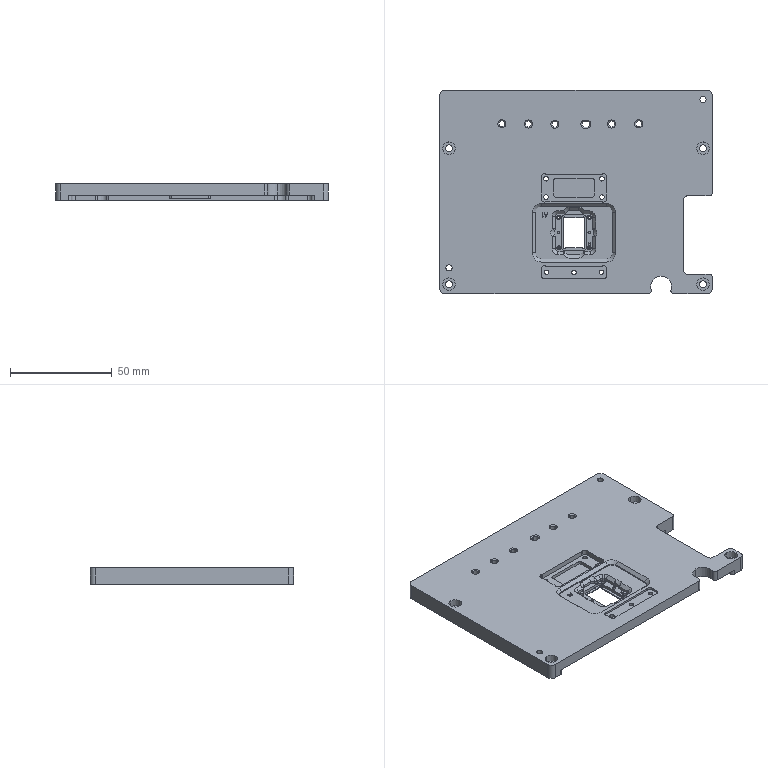NC program | NX | posted with a generic post | part box 134 x 100 x 8 mm
Lines 1 to 1315 of 16793:
N10 G17 G21 G94 G90
(FLOOR_WALL_COPY , TOOL : D63)
N12 T03 M6
N14 G54
N16 G17 G0 G90 X-105.5 Y53.999 S6500 M3
N18 G43 Z30. H3
N20 Z3.
N22 G94 G1 Z0. F1250.
N24 X-102.5
N26 X102.5
N28 Y12.6
N30 X-102.5
N32 Y-28.8
N34 X102.5
N36 X105.5
N38 Z3.
N40 G0 Z30.
N42 M5
(DRILLING_COPY_1 , TOOL : D6A45)
N44 T01 M6
N46 G54
N48 G17 G0 G90 X-62.5 Y-45.396 S5000 M3
N50 G43 Z30. H1
N52 G94 G81 G98 Z-0.5 F250. R3.
N54 Y-37.296
N56 Y21.5
N58 X-36.457 Y33.557
N60 X-23.437 Y33.443
N62 X-10.372 Y33.331
N64 X4.356
N66 X17.491 Y33.445
N68 X30.853 Y33.52
N70 X62.5 Y45.5
N72 Y21.5
N74 X12.75 Y6.5
N76 Y-2.5
N78 X-14.75 Y6.5
N80 Y-2.5
N82 X-8.5 Y-12.5
N84 X-5.7 Y-12.88
N86 X3.7
N88 X6.5 Y-12.5
N90 Y-27.5
N92 X3.7 Y-27.12
N94 X-5.7
N96 X-8.5 Y-27.5
N98 X-14.5 Y-39.5
N100 X-1.
N102 X12.5
N104 X62.5 Y-45.396
N106 G80
N108 G0 X62.5 Y-45.396 Z30.
N110 M5
(DRILLING_COPY_1_COPY , TOOL : 3.5ZT)
N112 T13 M6
N114 G54
N116 G17 G0 G90 X-62.5 Y21.5 S2000 M3
N118 G43 Z30. H13
N120 G94 G83 G98 Z-10.552 F150. Q2. R3.
N122 Y-45.396
N124 X62.5
N126 Y21.5
N128 G80
N130 G0 X62.5 Y21.5 Z30.
N132 M5
(DRILLING_COPY_1_COPY_COPY , TOOL : 2.2ZT)
N134 T12 M6
N136 G54
N138 G17 G0 G90 X-62.5 Y-37.296 S2000 M3
N140 G43 Z30. H12
N142 G94 G83 G98 Z-10.161 F150. Q2. R3.
N144 X-14.5 Y-39.5 Z-4.661
N146 X-1.
N148 X12.5
N150 X12.75 Y-2.5 Z-6.261
N152 Y6.5
N154 X-14.75 Y-2.5
N156 Y6.5
N158 X4.356 Y33.331 Z-7.661
N160 X62.5 Y45.5 Z-10.161
N162 G80
N164 G0 X62.5 Y45.5 Z30.
N166 M5
(DRILLING_COPY_1_COPY_COPY_COPY_2 , TOOL : 3.0ZT)
N168 T23 M6
N170 G54
N172 G17 G0 G90 X-36.457 Y33.557 S2000 M3
N174 G43 Z30. H23
N176 G94 G83 G98 Z-7.901 F150. Q2. R3.
N178 X-23.437 Y33.443
N180 X-10.372 Y33.331
N182 X17.491 Y33.445
N184 X30.853 Y33.52
N186 G80
N188 G0 X30.853 Y33.52 Z30.
N190 M5
(DRILLING_COPY_1_COPY_COPY_COPY , TOOL : 1.0ZT)
N192 T11 M6
N194 G54
N196 G17 G0 G90 X-8.5 Y-12.5 S3000 M3
N198 G43 Z30. H11
N200 G94 G83 G98 Z-8.9 F100. Q1. R3.
N202 X6.5
N204 Y-27.5
N206 X-8.5
N208 G80
N210 G0 X-8.5 Y-27.5 Z30.
N212 M5
(DRILLING_COPY_1_COPY_COPY_COPY_1 , TOOL : 1.2ZT)
N214 T20 M6
N216 G54
N218 G17 G0 G90 X3.7 Y-12.88 S3000 M3
N220 G43 Z30. H20
N222 G94 G83 G98 Z-8.611 F100. Q1. R3.
N224 X-5.7
N226 Y-27.12
N228 X3.7
N230 G80
N232 G0 X3.7 Y-27.12 Z30.
N234 M5
(ADAPTIVE_MILLING_COPY , TOOL : D10)
N236 T04 M6
N238 G54
N240 G17 G0 G90 X-78.709 Y-0.061 S9500 M3
N242 G43 Z30. H4
N244 Z-7.
N246 G94 G1 Z-8. F1000.
N248 X-77.928 Y-0.341 F3500.
N250 X-77.14 Y-0.597
N252 G3 X-76.062 Y-0.061 R1.017
N254 X-75.301 Y3.002 R8.28
N256 X-75.019 Y12.869 R111.643
N258 G1 X-75.014 Y15.119
N260 X-75.011 Y18.994
N262 X-75.01 Y32.619
N264 Y50.869
N266 X-75.009 Y50.994
N268 X-75.008 Y51.119
N270 G2 X-72.514 Y55.4 R5.714
N272 X-66.951 Y57.485 R12.445
N274 X-58.346 Y57.959 R64.172
N276 G1 X-57.221 Y57.968
N278 X-55.721 Y57.976
N280 X-53.846 Y57.982
N282 X-50.971 Y57.985
N284 X-45.096 Y57.987
N286 X68.029 Y57.988
N288 X68.154 Y57.986
N290 X68.279 Y57.979
N292 X68.404 Y57.968
N294 G2 X72.57 Y55.264 R5.937
N296 X74.529 Y49.65 R13.117
N298 X74.964 Y40.792 R70.999
N300 G1 X74.973 Y39.542
N302 X74.979 Y38.042
N304 X74.984 Y35.792
N306 X74.987 Y32.042
N308 X74.988 Y20.292
N310 Y-50.958
N312 G2 X72.718 Y-55.225 R5.577
N314 X67.211 Y-57.439 R11.915
N316 X59.11 Y-57.951 R54.383
N318 G1 X58.235 Y-57.96
N320 X56.985 Y-57.97
N322 X55.735 Y-57.976
N324 X53.86 Y-57.982
N326 X50.86 Y-57.986
N328 X44.36 Y-57.987
N330 X-68.015 Y-57.988
N332 X-68.14 Y-57.986
N334 X-68.265 Y-57.979
N336 X-68.389 Y-57.969
N338 G2 X-72.56 Y-55.274 R5.92
N340 X-74.527 Y-49.661 R13.075
N342 X-74.964 Y-40.804 R70.368
N344 G1 X-74.973 Y-39.554
N346 X-74.979 Y-37.929
N348 X-74.984 Y-35.554
N350 X-74.987 Y-31.554
N352 X-74.988 Y-16.679
N354 Y-3.804
N356 G2 X-74.49 Y1.42 R59.156
N358 G3 X-74.037 Y13.656 R126.306
N360 G1 X-74.031 Y15.406
N362 X-74.025 Y17.906
N364 X-74.022 Y21.906
N366 X-74.021 Y32.906
N368 Y47.906
N370 X-74.019 Y48.031
N372 G2 X-70.421 Y54.267 R7.625
N374 X-64.091 Y56.445 R15.186
N376 X-55.111 Y56.94 R70.872
N378 G1 X-53.986 Y56.951
N380 X-52.611 Y56.96
N382 X-50.861 Y56.967
N384 X-48.486 Y56.972
N386 X-44.611 Y56.976
N388 X-33.111 Y56.977
N390 X64.889
N392 X65.139 Y56.975
N394 X65.264 Y56.97
N396 X65.389 Y56.964
N398 G2 X71.397 Y53.191 R7.687
N400 X73.483 Y46.827 R15.724
N402 X73.952 Y36.844 R83.323
N404 G1 X73.962 Y35.344
N406 X73.969 Y33.344
N408 X73.974 Y30.844
N410 X73.977 Y26.344
N412 Y5.594
N414 X73.978 Y-30.031
N416 X73.984 Y-31.656
N418 X73.983 Y-33.031
N420 X73.987 Y-34.031
N422 X73.984 Y-35.531
N424 X73.987 Y-36.406
N426 X73.986 Y-37.406
N428 X73.989 Y-38.656
N430 X73.987 Y-39.656
N432 X73.988 Y-40.406
N434 X73.987 Y-41.531
N436 X73.986 Y-42.156
N438 X73.988 Y-43.031
N440 X73.986 Y-44.281
N442 X73.988 Y-45.156
N444 X73.987 Y-46.281
N446 X73.99 Y-47.531
N448 X73.989 Y-47.906
N450 X73.986 Y-48.156
N452 X73.981 Y-48.28
N454 X73.974 Y-48.405
N456 G2 X70.182 Y-54.403 R7.71
N458 X63.941 Y-56.47 R15.659
N460 X54.459 Y-56.947 R77.622
N462 G1 X53.209 Y-56.957
N464 X51.584 Y-56.965
N466 X49.584 Y-56.97
N468 X46.459 Y-56.975
N470 X40.334 Y-56.977
N472 X-64.916
N474 X-65.041 Y-56.976
N476 X-65.166 Y-56.973
N478 X-65.291 Y-56.968
N480 X-65.416 Y-56.962
N482 X-65.54 Y-56.953
N484 G2 X-71.411 Y-53.165 R7.74
N486 X-73.503 Y-46.673 R15.948
N488 X-73.956 Y-36.439 R88.425
N490 G1 X-73.964 Y-34.939
N492 X-73.97 Y-33.064
N494 X-73.974 Y-30.314
N496 X-73.977 Y-25.314
N498 Y-6.189
N500 X-73.975 Y-5.814
N502 G2 X-73.436 Y2.041 R136.426
N504 G3 X-73.042 Y17.282 R216.987
N506 G1 X-73.037 Y19.907
N508 X-73.033 Y23.907
N510 X-73.031 Y33.407
N512 Y44.907
N514 X-73.029 Y45.282
N516 X-73.028 Y45.407
N518 G2 X-71.472 Y50.593 R8.925
N520 X-70.439 Y52.312 R10.087
N522 X-67.763 Y54.412 R8.758
N524 X-63.801 Y55.355 R14.165
N526 X-52.823 Y55.929 R91.403
N528 G1 X-51.698 Y55.939
N530 X-50.198 Y55.948
N532 X-48.323 Y55.956
N534 X-45.823 Y55.961
N536 X-41.823 Y55.965
N538 X-31.948 Y55.966
N540 X62.302
N542 X62.552 Y55.963
N544 X62.677 Y55.961
N546 X62.927 Y55.953
N548 X63.052 Y55.947
N550 G2 X67.462 Y54.517 R8.648
N552 G1 X67.763 Y54.412
N554 X67.87 Y54.361
N556 G2 X70.513 Y52.219 R8.758
N558 X72.187 Y47.913 R8.812
N560 X72.917 Y36.948 R74.282
N562 G1 X72.93 Y35.823
N564 X72.941 Y34.573
N566 X72.949 Y33.073
N568 X72.957 Y31.198
N570 X72.962 Y28.573
N572 X72.965 Y24.448
N574 X72.967 Y13.698
N576 Y-26.927
N578 X72.974 Y-28.302
N580 X72.975 Y-30.052
N582 X72.978 Y-30.802
N584 X72.98 Y-31.927
N586 G2 X72.958 Y-46.177 R809.535
N588 X71.503 Y-50.503 R8.675
N590 X70.439 Y-52.312 R8.604
N592 X67.763 Y-54.412 R8.758
N594 X63.801 Y-55.355 R14.165
N596 X52.823 Y-55.93 R91.279
N598 G1 X51.573 Y-55.94
N600 X50.073 Y-55.949
N602 X48.073 Y-55.956
N604 X45.448 Y-55.962
N606 X41.198 Y-55.965
N608 X29.198 Y-55.966
N610 X-62.302
N612 X-62.427 Y-55.965
N614 X-62.552 Y-55.963
N616 X-62.802 Y-55.956
N618 X-62.927 Y-55.951
N620 X-63.052 Y-55.945
N622 G2 X-67.453 Y-54.52 R8.649
N624 G1 X-67.763 Y-54.412
N626 X-67.87 Y-54.361
N628 G2 X-70.513 Y-52.219 R8.758
N630 X-72.187 Y-47.913 R8.812
N632 X-72.908 Y-37.572 R72.544
N634 X-72.966 Y-22.073 R825.905
N636 X-72.913 Y-5.323 R785.834
N638 G1 X-72.893 Y-4.824
N640 X-72.869 Y-4.324
N642 X-72.841 Y-3.825
N644 X-72.81 Y-3.326
N646 X-72.759 Y-2.578
N648 X-72.688 Y-1.58
N650 X-72.597 Y-0.334
N652 X-72.498 Y1.163
N654 X-72.401 Y2.66
N656 X-72.358 Y3.409
N658 X-72.326 Y4.033
N660 X-72.297 Y4.657
N662 X-72.26 Y5.531
N664 X-72.227 Y6.406
N666 X-72.198 Y7.28
N668 X-72.177 Y8.03
N670 X-72.154 Y8.905
N672 X-72.15 Y9.087
N674 Y47.47
N676 X-72.147 Y47.53
N678 X-71.965 Y49.143
N680 X-71.938 Y49.259
N682 X-71.443 Y50.674
N684 G2 X-69.219 Y53.513 R8.407
N686 X-66.143 Y54.965 R8.758
N688 G1 X-64.53 Y55.147
N690 X-64.47 Y55.15
N692 X64.47
N694 X64.53 Y55.147
N696 X66.143 Y54.965
N698 X66.259 Y54.938
N700 X67.556 Y54.484
N702 X67.87 Y54.361
N704 G2 X70.513 Y52.219 R8.758
N706 X71.965 Y49.143 R8.758
N708 G1 X72.147 Y47.53
N710 X72.15 Y47.47
N712 Y-0.401
N714 G3 X71.979 Y-14.083 R281.781
N716 G1 X71.978 Y-23.833
N718 Y-40.458
N720 X71.983 Y-40.513
N722 X71.99 Y-40.544
N724 X72.147 Y-41.935
N726 X72.15 Y-41.994
N728 Y-47.47
N730 X72.147 Y-47.53
N732 X71.965 Y-49.143
N734 X71.938 Y-49.259
N736 X71.484 Y-50.556
N738 G3 X73.623 Y-50.935 R-1.1
N740 G1 X73.776 Y-40.187
N742 X73.804 Y-38.187 Z-7.9
N744 X74.308 Y-2.823
N746 X74.336 Y-0.823 Z-8.
N748 G3 X74.131 Y0.061 R1.327
N750 X72.147 Y-0.461 R1.101
N752 G2 X71.621 Y-3.038 R8.661
N754 G3 X71.061 Y-9.127 R31.238
N756 X70.989 Y-24.377 R776.181
N758 G1 Y-37.877
N760 Y-38.002
N762 X71.002 Y-38.126
N764 G3 X71.511 Y-39.135 R3.65
N766 G1 X71.964 Y-40.428
N768 X71.99 Y-40.544
N770 G3 X73.845 Y-41.071 R1.102
N772 X74.161 Y-40.102 Z-7.947 R1.227
N774 G1 X74.154 Y-39.155 Z-7.9
N776 X73.903 Y-4.015
N778 Y-3.374 Z-7.932
N780 X73.879 Y-2.734 Z-7.964
N782 G3 X73.543 Y-2.114 Z-8. R1.143
N784 X71.757 Y-2.557 R1.102
N786 G2 X71.062 Y-4.145 R11.213
N788 G3 X70.204 Y-9.179 R17.999
N790 X70.004 Y-21.301 R238.834
N792 X70.029 Y-36.425 R855.256
N794 X70.657 Y-37.776 R1.574
N796 G1 X70.731 Y-37.869
N798 X71.13 Y-38.504
N800 G3 X72.608 Y-38.873 R1.104
N802 X73.162 Y-37.83 Z-7.938 R1.124
N804 G1 X73.166 Y-37.074 Z-7.9
N806 X73.353 Y-5.053
N808 X73.347 Y-4.011 Z-7.952
N810 G3 X72.843 Y-3.232 Z-8. R1.117
N812 X71.327 Y-3.579 R1.104
N814 X69.531 Y-8.312 R9.834
N816 X69.046 Y-17.542 R72.207
N818 X69.055 Y-35.041 R637.354
N820 X69.372 Y-36.492 R3.287
N822 G1 X69.448 Y-36.592
N824 X69.533 Y-36.684
N826 X69.578 Y-36.722
N828 X69.596 Y-36.733
N830 X69.688 Y-36.807
N832 X70.395 Y-37.514
N834 G3 X71.725 Y-37.688 R1.108
N836 X72.274 Y-36.655 Z-7.938 R1.125
N838 G1 X72.285 Y-35.887 Z-7.9
N840 X72.679 Y-6.107
N842 X72.681 Y-5.068 Z-7.952
N844 G3 X72.181 Y-4.284 Z-8. R1.117
N846 X70.731 Y-4.527 R1.106
N848 X69.01 Y-7.65 R6.182
N850 X68.163 Y-14.836 R33.413
N852 X68.073 Y-33.709 R409.302
N854 X68.585 Y-36.005 R5.128
N856 X69.596 Y-36.733 R3.984
N858 X70.75 Y-36.743 R1.112
N860 X71.286 Y-35.654 Z-7.936 R1.183
N862 G1 X71.307 Y-34.932 Z-7.9
N864 X72.154 Y-6.662
N866 X72.174 Y-5.624 Z-7.952
N868 G3 X71.685 Y-4.831 Z-8. R1.117
N870 X70.303 Y-4.973 R1.106
N872 X68.11 Y-8.666 R6.798
N874 X67.213 Y-15.72 R32.889
N876 X67.099 Y-32.592 R281.712
N878 X67.726 Y-35.503 R7.4
N880 X68.436 Y-36.004 R1.472
N882 G1 X68.859 Y-36.271
N884 G3 X70.057 Y-36.253 R1.111
N886 X70.547 Y-35.279 Z-7.943 R1.132
N888 G1 X70.575 Y-34.417 Z-7.9
N890 X71.445 Y-7.381
N892 X71.467 Y-6.326 Z-7.953
N894 G3 X70.996 Y-5.541 Z-8. R1.117
N896 X69.688 Y-5.588 R1.108
N898 X67.704 Y-8.074 R4.795
N900 X66.404 Y-14.417 R21.662
N902 X66.061 Y-26.534 R167.955
N904 X66.273 Y-33.025 R47.803
N906 X67.075 Y-35.367 R5.249
N908 X68.288 Y-35.939 R2.889
N910 X69.303 Y-35.786 R1.116
N912 X69.758 Y-34.763 Z-7.942 R1.202
N914 G1 X69.794 Y-33.931 Z-7.9
N916 X70.922 Y-7.779
N918 X70.949 Y-7.222 Z-7.928
N920 X70.956 Y-6.664 Z-7.956
N922 G3 X70.529 Y-5.917 Z-8. R1.128
N924 X69.278 Y-5.862 R1.108
N926 X66.876 Y-8.634 R5.157
N928 X65.496 Y-14.833 R21.41
N930 X65.149 Y-30.57 R145.818
N932 X65.959 Y-34.59 R11.113
N934 X67.036 Y-35.501 R1.403
N936 G1 X67.508 Y-35.666
N938 G3 X68.6 Y-35.451 R1.112
N940 X68.979 Y-34.491 Z-7.947 R1.22
N942 G1 X69.021 Y-33.56 Z-7.9
N944 X70.178 Y-8.255
N946 X70.207 Y-7.695 Z-7.928
N948 X70.215 Y-7.134 Z-7.956
N950 G3 X69.797 Y-6.389 Z-8. R1.128
N952 X68.537 Y-6.327 R1.108
N954 X66.31 Y-8.578 R4.465
N956 X64.687 Y-14.452 R17.91
N958 X64.118 Y-25.556 R98.682
N960 X64.502 Y-32.408 R34.226
N962 X65.688 Y-35.122 R5.464
N964 X66.92 Y-35.474 R2.043
N966 X67.794 Y-35.186 R1.117
N968 X68.153 Y-34.255 Z-7.949 R1.24
N970 G1 X68.213 Y-33.285 Z-7.9
N972 X69.73 Y-8.539
N974 X69.768 Y-7.96 Z-7.929
N976 X69.788 Y-7.38 Z-7.958
N978 G3 X69.414 Y-6.651 Z-8. R1.129
N980 X68.329 Y-6.442 R1.112
N982 X65.769 Y-8.497 R4.142
N984 X63.915 Y-14.035 R15.663
N986 X63.176 Y-24.124 R71.005
N988 X63.488 Y-31.481 R40.611
N990 X64.765 Y-34.836 R7.471
N992 X65.53 Y-35.318 R1.293
N994 G1 X66.275 Y-35.402
N996 G3 X67.242 Y-35.014 R1.115
N998 X67.508 Y-34.174 Z-7.955 R1.288
N1000 G1 X67.573 Y-33.077 Z-7.9
N1002 X69.019 Y-8.85
N1004 X69.081 Y-7.637 Z-7.961
N1006 G3 X68.753 Y-6.942 Z-8. R1.133
N1008 X67.621 Y-6.69 R1.111
N1010 X64.965 Y-8.82 R4.429
N1012 X63.012 Y-14.455 R15.931
N1014 X62.207 Y-26.414 R70.313
N1016 X62.931 Y-32.601 R22.558
N1018 X64.322 Y-35.076 R5.317
N1020 X65.53 Y-35.318 R1.843
N1022 X66.457 Y-34.898 R1.116
N1024 X66.701 Y-34.099 Z-7.957 R1.288
N1026 G1 X66.775 Y-32.954 Z-7.9
N1028 X68.31 Y-9.104
N1030 X68.378 Y-7.883 Z-7.961
N1032 G3 X68.061 Y-7.191 Z-8. R1.133
N1034 X67.036 Y-6.895 R1.113
N1036 X64.754 Y-8.285 R3.478
N1038 X62.431 Y-13.357 R12.694
N1040 X61.335 Y-22.401 R47.087
N1042 X61.657 Y-30.753 R38.849
N1044 X63.2 Y-34.669 R8.88
N1046 X64.213 Y-35.314 R1.515
N1048 G1 X64.963
N1050 G3 X65.867 Y-34.841 R1.116
N1052 X66.074 Y-34.108 Z-7.961 R1.319
N1054 G1 X66.165 Y-32.885 Z-7.9
N1056 X67.932 Y-9.239
N1058 X67.985 Y-8.588 Z-7.933
N1060 X68.016 Y-7.937 Z-7.965
N1062 G3 X67.75 Y-7.307 Z-8. R1.145
N1064 X66.796 Y-6.935 R1.116
N1066 X64.106 Y-8.328 R3.633
N1068 X61.671 Y-13.207 R12.269
N1070 X60.398 Y-22.476 R42.933
N1072 X60.797 Y-30.697 R35.141
N1074 X62.47 Y-34.693 R9.032
N1076 X63.467 Y-35.314 R1.555
N1078 G1 X64.217
N1080 G3 X65.154 Y-34.789 R1.112
N1082 X65.329 Y-34.105 Z-7.964 R1.401
N1084 G1 X65.431 Y-32.824 Z-7.9
N1086 X67.299 Y-9.391
N1088 X67.356 Y-8.71 Z-7.934
N1090 X67.396 Y-8.028 Z-7.968
N1092 G3 X67.181 Y-7.442 Z-8. R1.153
N1094 X66.175 Y-7.005 R1.112
N1096 X63.348 Y-8.456 R3.873
N1098 X60.737 Y-13.661 R12.874
N1100 X59.696 Y-29.29 R43.796
N1102 X61.345 Y-34.229 R11.874
N1104 X62.536 Y-35.285 R2.336
N1106 G1 X62.658 Y-35.309
N1108 X62.698 Y-35.314
N1110 X63.573
N1112 G3 X64.511 Y-34.789 R1.112
N1114 X64.685 Y-34.102 Z-7.964 R1.398
N1116 G1 X64.784 Y-32.824 Z-7.9
N1118 X66.594 Y-9.476
N1120 X66.649 Y-8.791 Z-7.934
N1122 X66.689 Y-8.105 Z-7.969
N1124 G3 X66.478 Y-7.526 Z-8. R1.154
N1126 X65.53 Y-7.078 R1.115
N1128 X63.011 Y-8.131 R3.402
N1130 X60.164 Y-12.916 R11.458
N1132 X58.552 Y-22.628 R36.328
N1134 X59.166 Y-30.952 R29.441
N1136 X61.06 Y-34.844 R8.753
N1138 X61.92 Y-35.314 R1.439
N1140 G1 X62.795
N1142 G3 X63.733 Y-34.788 R1.112
N1144 X63.908 Y-34.113 Z-7.965 R1.414
N1146 G1 X64.022 Y-32.823 Z-7.9
N1148 X66.08 Y-9.539
N1150 X66.194 Y-8.131 Z-7.971
N1152 G3 X66.016 Y-7.579 Z-8. R1.162
N1154 X65.095 Y-7.081 R1.115
N1156 X62.272 Y-8.183 R3.653
N1158 X59.355 Y-12.928 R11.64
N1160 X58.232 Y-17.292 R28.131
N1162 X58.259 Y-29.541 R751.286
N1164 X60.101 Y-34.639 R9.31
N1166 X61.148 Y-35.314 R1.666
N1168 G1 X62.023
N1170 G3 X62.999 Y-33.707 R1.102
N1172 G1 X60.308 Y-28.534
N1174 G3 X58.232 Y-29.042 R1.101
N1176 X58.322 Y-32.161 R20.278
N1178 X59.866 Y-35.093 R5.132
N1180 X60.445 Y-35.314 R1.906
N1182 G1 X61.195
N1184 G3 X62.123 Y-33.623 R1.102
N1186 G1 X60.26 Y-30.7
N1188 G3 X58.232 Y-31.292 R1.101
N1190 X58.364 Y-33.529 R8.555
N1192 X59.426 Y-35.175 R2.884
N1194 X60.51 Y-35.314 R2.217
N1196 X61.385 Y-33.548 R1.101
N1198 G1 X60.208 Y-32.
N1200 G3 X58.232 Y-32.667 R1.101
N1202 X58.455 Y-34.509 R4.147
N1204 X59.984 Y-35.314 R1.385
N1206 X60.774 Y-33.449 R1.101
N1208 G1 X60.39 Y-33.048
N1210 X59.992 Y-32.661
N1212 G3 X58.232 Y-33.542 R1.101
N1214 X58.391 Y-34.767 R2.554
N1216 X59.496 Y-35.314 R1.196
N1218 X59.64 Y-33.088 R1.119
N1220 X58.285 Y-34.511 R1.191
N1222 X60.2 Y-34.857 R1.093
N1224 G1 X60.292 Y-34.708
N1226 X60.401 Y-34.388 Z-7.983
N1228 X60.466 Y-34.056 Z-7.966
N1230 X60.728 Y-32.76 Z-7.9
N1232 X65.408 Y-9.598
N1234 X65.674 Y-8.227 Z-7.97
N1236 G3 X65.545 Y-7.646 Z-8. R1.137
N1238 X64.595 Y-7.081 R1.093
N1240 X61.433 Y-8.296 R3.958
N1242 X58.232 Y-13.907 R12.411
N1244 G1 Y-17.407
N1246 G3 X59.478 Y-18.497 R1.103
N1248 X60.401 Y-17.725 Z-7.937 R1.188
N1250 G1 X60.724 Y-17.065 Z-7.9
N1252 X64.378 Y-9.595
N1254 X64.643 Y-9.059 Z-7.93
N1256 X64.893 Y-8.516 Z-7.96
N1258 G3 X64.849 Y-7.731 Z-8. R1.131
N1260 X63.845 Y-7.081 R1.111
N1262 X60.777 Y-8.229 R4.002
N1264 X58.265 Y-11.767 R10.358
N1266 X58.232 Y-13.944 R25.502
N1268 X59.259 Y-15.042 R1.104
N1270 X60.297 Y-14.481 Z-7.938 R1.124
N1272 G1 X60.72 Y-13.853 Z-7.9
N1274 X63.592 Y-9.596
N1276 X63.913 Y-9.127 Z-7.928
N1278 X64.217 Y-8.646 Z-7.957
N1280 G3 X64.254 Y-7.807 Z-8. R1.128
N1282 X63.22 Y-7.081 R1.108
N1284 X59.932 Y-8.317 R4.189
N1286 X58.291 Y-10.346 R7.232
N1288 X58.232 Y-11.985 R7.202
N1290 X60.181 Y-12.685 R1.101
N1292 G1 X63.319 Y-8.881
N1294 G3 X62.47 Y-7.081 R1.101
N1296 X59.176 Y-8.311 R4.251
N1298 X58.24 Y-9.601 R2.456
N1300 G1 X58.232 Y-9.66
N1302 Y-10.66
N1304 G3 X60.124 Y-11.424 R1.101
N1306 G1 X62.512 Y-8.944
N1308 G3 X61.72 Y-7.081 R1.101
N1310 X58.399 Y-8.464 R3.81
N1312 X58.232 Y-9.71 R2.337
N1314 X60.083 Y-10.514 R1.101
N1316 G1 X61.721 Y-8.985
N1318 G3 X60.97 Y-7.081 R1.101
N1320 X58.532 Y-7.805 R3.17
N1322 X58.232 Y-8.979 R1.536
N1324 X60.067 Y-9.797 R1.101
N1326 G1 X60.58 Y-9.343
N1328 X61.077 Y-8.871
N1330 G3 X60.22 Y-7.081 R1.101
N1332 X58.659 Y-7.387 R2.465
N1334 X58.232 Y-8.596 R1.351
N1336 X60.261 Y-9.185 R1.101
N1338 G1 X60.608 Y-8.611
N1340 G3 X59.595 Y-7.081 R1.102
N1342 X58.252 Y-8.069 R1.17
N1344 X58.638 Y-8.996 R1.011
N1346 G1 X59.136 Y-9.374
N1348 X60.728 Y-10.585 Z-7.9
N1350 X61.259 Y-11.003
N1352 X61.434 Y-11.251
N1354 X72.055 Y-32.494
N1356 G2 X74.291 Y-37.866 R41.94
N1358 X75.324 Y-46.167 R22.043
N1360 G1 X75.117 Y-48.258
N1362 X74.872 Y-50.346
N1364 G2 X72.323 Y-55.086 R8.418
N1366 G1 X70.04 Y-57.215
N1368 G2 X68.603 Y-57.139 R1.004
N1370 G1 X68.364 Y-56.864
N1372 X67.054 Y-55.353 Z-8.
N1374 G3 X66.143 Y-54.965 R1.021
N1376 G1 X64.53 Y-55.147
N1378 X64.47 Y-55.15
N1380 X48.226
N1382 X47.912 Y-55.131
N1384 G3 X36.952 Y-54.979 R251.45
N1386 G1 X35.587 Y-55.146
N1388 X35.522 Y-55.15
N1390 X-64.47
N1392 X-64.53 Y-55.147
N1394 X-66.143 Y-54.965
N1396 X-66.259 Y-54.938
N1398 X-67.556 Y-54.484
N1400 G3 X-67.927 Y-56.623 R-1.1
N1402 G1 X36.05 Y-57.264
N1404 X38.05 Y-57.276 Z-7.9
N1406 X45.824 Y-57.324
N1408 X47.824 Y-57.337 Z-8.
N1410 G3 X48.81 Y-57.012 R1.236
N1412 X48.162 Y-55.146 R1.101
N1414 G2 X45.583 Y-54.621 R8.785
N1416 G3 X39.246 Y-54.084 R28.952
N1418 X38.601 Y-54.403 R3.083
N1420 G2 X36.843 Y-54.993 R7.726
N1422 G3 X36.43 Y-57.04 R1.101
N1424 X37.208 Y-57.178 Z-7.96 R1.331
N1426 G1 X38.404 Y-57.143 Z-7.9
N1428 X44.817 Y-56.955
N1430 X45.402 Y-56.94 Z-7.929
N1432 X45.987 Y-56.908 Z-7.959
N1434 G3 X46.674 Y-56.48 Z-8. R1.13
N1436 X46.182 Y-54.798 R1.103
N1438 G2 X44.12 Y-53.941 R65.155
N1440 G3 X40.309 Y-53.364 R11.346
N1442 G1 X40.187 Y-53.392
N1444 X40.068 Y-53.432
N1446 X39.955 Y-53.484
N1448 X39.932 Y-53.496
N1450 X38.803 Y-54.281
N1452 G3 X39.418 Y-56.284 R1.101
N1454 G1 X44.392 Y-56.346
N1456 G3 X45.034 Y-54.343 R1.101
N1458 X41.279 Y-52.81 R6.805
N1460 X40.028 Y-53.41 R1.334
N1462 G1 X39.932 Y-53.496
N1464 X39.83 Y-53.567
N1466 G3 X40.409 Y-55.569 R1.101
N1468 G1 X43.434 Y-55.702
N1470 G3 X44.11 Y-53.7 R1.101
N1472 G1 X43.816 Y-53.496
N1474 X43.72 Y-53.41
N1476 X43.638 Y-53.316
N1478 X43.548 Y-53.23
N1480 X43.453 Y-53.148
N1482 X43.354 Y-53.072
N1484 X43.253 Y-52.999
N1486 X43.148 Y-52.931
N1488 G3 X41.006 Y-52.49 R2.739
N1490 X40.213 Y-53.199 R2.279
N1492 X40.967 Y-55.022 R1.101
N1494 G1 X42.739 Y-55.139
N1496 G3 X43.638 Y-53.316 R1.101
N1498 X41.683 Y-52.116 R2.735
N1500 X40.558 Y-52.806 R1.455
N1502 X41.341 Y-54.63 R1.101
N1504 G1 X41.933 Y-54.657
N1506 X42.525 Y-54.665
N1508 G3 X43.226 Y-52.847 R1.101
N1510 X41.941 Y-51.927 R2.131
N1512 X41.227 Y-52.106 R1.312
N1514 X41.744 Y-54.038 R1.441
N1516 G1 Z-5.
N1518 G0 Z30.
N1520 X41.814 Y-54.109
N1522 Z-7.
N1524 G1 Z-8. F1000.
N1526 G3 X42.814 Y-52.377 R1.076 F3500.
N1528 X40.841 Y-52.484 R1.179
N1530 X40.703 Y-53.623 R1.052
N1532 G1 X41.393 Y-55.5 Z-7.9
N1534 G2 X41.483 Y-56.319 R1.201
N1536 X40.841 Y-56.984 R1.015
N1538 G1 X39.776 Y-57.34
N1540 X38.697 Y-57.652
N1542 G2 X36.608 Y-57.968 R14.971
N1544 X32.877 Y-58.185 R43.305
N1546 G1 X-47.121 Y-59.203
N1548 G2 X-60.832 Y-58.565 R116.885
N1550 G1 X-65.804 Y-58.037
N1552 G2 X-70.72 Y-56.195 R10.763
N1554 X-72.363 Y-54.851 R12.557
N1556 G1 X-74.215 Y-53.04
N1558 G2 X-74.157 Y-51.557 R1.004
N1560 G1 X-73.886 Y-51.331
N1562 X-72.35 Y-50.05 Z-8.
N1564 G3 X-71.965 Y-49.143 R1.017
N1566 G1 X-72.147 Y-47.53
N1568 X-72.15 Y-47.47
N1570 Y9.155
N1572 G3 X-73.001 Y10.152 R1.016
N1574 G1 X-74.569 Y10.403
N1576 Z-5.
N1578 G0 Z30.
(CAVITY_MILL , TOOL : D10)
N1580 X-5.805 Y3.7
N1582 Z1.5
N1584 G1 X-11.95 Z1.178 F1000.
N1586 Y0.3 Z1.
N1588 X9.95 Z-0.148
N1590 Y3.7 Z-0.326
N1592 X-1. Z-0.9
N1594 X-11.95 F3000.
N1596 Y0.3
N1598 X9.95
N1600 Y3.7
N1602 X-1.
N1604 G3 X-1.866 Y3.2 R1.
N1606 G1 Z0.6
N1608 G0 Z30.
N1610 X-3.897 Y3.7
N1612 Z0.6
N1614 G1 X-11.95 Z0.178 F1000.
N1616 Y0.3 Z0.
N1618 X9.95 Y0.301 Z-1.148
N1620 Y3.7 Z-1.326
N1622 X-1. Z-1.9
N1624 X-11.95 F3000.
N1626 Y0.3
N1628 X9.95 Y0.301
N1630 Y3.7
N1632 X-1.
N1634 G3 X-1.866 Y3.2 R1.
N1636 G1 Z-0.4
N1638 G0 X-6.23 Y0.3
N1640 G1 X9.95 Y0.301 Z-1.248 F1000.
N1642 Y3.7 Z-1.426
N1644 X-1. Z-2.
N1646 X-11.95 F3000.
N1648 Y0.3
N1650 X9.95 Y0.301
N1652 Y3.7
N1654 X-1.
N1656 G3 X-1.866 Y3.2 R1.
N1658 G1 Z-0.5
N1660 G0 X-11.95 Y2.213
N1662 G1 Y0.3 Z-0.6 F1000.
N1664 X9.95 Y0.301 Z-1.748
N1666 Y3.7 Z-1.926
N1668 X-1. Z-2.5
N1670 X-11.95 F3000.
N1672 Y0.3
N1674 X9.95 Y0.301
N1676 Y3.7
N1678 X-1.
N1680 G3 X-1.866 Y3.2 R1.
N1682 G1 Z-1.
N1684 G0 Z30.
N1686 X-8.466 Y-18.866
N1688 Z1.5
N1690 G1 Y-21.466 Z1.364 F1000.
N1692 X6.466 Z0.581
N1694 Y-18.534 Z0.428
N1696 X-8.466 Z-0.355
N1698 Y-21.466 Z-0.509
N1700 X-1. Z-0.9
N1702 X6.466 F3000.
N1704 Y-18.534
N1706 X-8.466
N1708 Y-21.466
N1710 X-1.
N1712 Y-28.466
N1714 X13.466
N1716 Y-11.534
N1718 X-15.466
N1720 Y-28.466
N1722 X-1.
N1724 G3 X-0.134 Y-27.966 R1.
N1726 G1 Z0.6
N1728 G0 Z30.
N1730 X-0.097 Y-19.1
N1732 Z0.6
N1734 G1 X-7.9 Z0.191 F1000.
N1736 Y-20.9 Z0.097
N1738 X5.9 Z-0.626
N1740 Y-19.1 Z-0.721
N1742 X-7.9 Z-1.444
N1744 Y-20.9 Z-1.538
N1746 X-1. Z-1.9
N1748 X5.9 F3000.
N1750 Y-19.1
N1752 X-7.9
N1754 Y-20.9
N1756 X-1.
N1758 Y-27.9
N1760 X12.9
N1762 Y-12.1
N1764 X-14.9
N1766 Y-27.9
N1768 X-1.
N1770 G3 X-0.134 Y-27.4 R1.
N1772 G1 Z-0.4
N1774 G0 X-1.303 Y-22.441
N1776 G1 X-1. Y-22.631 Z-0.419 F1000.
N1778 X-0.438 Y-22.28 Z-0.453
N1780 X0.166 Y-22.009 Z-0.488
N1782 X0.164 Y-21.248 Z-0.528
N1784 X0.216 Y-20.745 Z-0.555
N1786 X0.372 Y-20. Z-0.594
N1788 X0.216 Y-19.255 Z-0.634
N1790 X0.166 Y-18.778 Z-0.659
N1792 Y-17.991 Z-0.701
N1794 X-0.438 Y-17.72 Z-0.735
N1796 X-1. Y-17.369 Z-0.77
N1798 X-1.562 Y-17.72 Z-0.805
N1800 X-2.166 Y-17.991 Z-0.84
N1802 X-2.164 Y-18.752 Z-0.879
N1804 X-2.216 Y-19.255 Z-0.906
N1806 X-2.372 Y-20. Z-0.946
N1808 X-2.216 Y-20.745 Z-0.986
N1810 X-2.166 Y-21.222 Z-1.011
N1812 Y-22.009 Z-1.052
N1814 X-1.562 Y-22.28 Z-1.087
N1816 X-1. Y-22.631 Z-1.122
N1818 X-0.438 Y-22.28 Z-1.156
N1820 X0.166 Y-22.009 Z-1.191
N1822 X0.164 Y-21.248 Z-1.231
N1824 X0.216 Y-20.745 Z-1.257
N1826 X0.372 Y-20. Z-1.297
N1828 X0.216 Y-19.255 Z-1.337
N1830 X0.166 Y-18.778 Z-1.362
N1832 Y-17.991 Z-1.403
N1834 X-0.438 Y-17.72 Z-1.438
N1836 X-1. Y-17.369 Z-1.473
N1838 X-1.562 Y-17.72 Z-1.508
N1840 X-2.166 Y-17.991 Z-1.542
N1842 X-2.164 Y-18.752 Z-1.582
N1844 X-2.216 Y-19.255 Z-1.609
N1846 X-2.372 Y-20. Z-1.649
N1848 X-2.216 Y-20.745 Z-1.688
N1850 X-2.166 Y-21.222 Z-1.714
N1852 Y-22.009 Z-1.755
N1854 X-1.562 Y-22.28 Z-1.79
N1856 X-1. Y-22.631 Z-1.824
N1858 X-0.438 Y-22.28 Z-1.859
N1860 X0.166 Y-22.009 Z-1.894
N1862 X0.164 Y-21.248 Z-1.934
N1864 X0.216 Y-20.745 Z-1.96
N1866 X0.372 Y-20. Z-2.
N1868 G2 X0.166 Y-17.991 R9.634 F3000.
N1870 X-1. Y-17.369 R9.634
N1872 X-2.166 Y-17.991 R9.634
N1874 X-2.372 Y-20. R9.634
N1876 X-2.166 Y-22.009 R9.634
N1878 X-1. Y-22.631 R9.634
N1880 X0.166 Y-22.009 R9.634
N1882 X0.372 Y-20. R9.634
N1884 G1 X4.776 Y-20.926
N1886 G2 X5.065 Y-20. R5.134
N1888 X4.666 Y-18.017 R5.134
N1890 G1 Y-14.334
N1892 X4.107
N1894 G2 X0.29 Y-12.634 R5.134
N1896 G1 X-2.29
N1898 G2 X-6.107 Y-14.334 R5.134
N1900 G1 X-6.666
N1902 Y-18.017
N1904 G2 X-7.065 Y-19.999 R5.134
N1906 X-6.666 Y-21.983 R5.134
N1908 G1 Y-25.666
N1910 X-6.107
N1912 G2 X-2.29 Y-27.366 R5.134
N1914 G1 X0.29
N1916 G2 X4.107 Y-25.666 R5.134
N1918 G1 X4.666
N1920 Y-21.983
N1922 G2 X4.776 Y-20.926 R5.134
N1924 G3 X4.465 Y-19.976 R1.
N1926 G1 Z-0.5
N1928 G0 X4.166 Y-15.687
N1930 G1 Y-14.834 Z-0.545 F1000.
N1932 X3.524 Z-0.578
N1934 X2.431 Y-14.611 Z-0.637
N1936 X1.403 Y-14.177 Z-0.695
N1938 X0.48 Y-13.551 Z-0.754
N1940 X0.074 Y-13.134 Z-0.784
N1942 X-2.074 Z-0.897
N1944 X-2.48 Y-13.551 Z-0.927
N1946 X-3.403 Y-14.177 Z-0.986
N1948 X-4.431 Y-14.611 Z-1.044
N1950 X-5.524 Y-14.834 Z-1.103
N1952 X-6.166 Z-1.136
N1954 Y-18.599 Z-1.334
N1956 X-6.322 Y-19.455 Z-1.379
N1958 X-6.527 Y-20. Z-1.41
N1960 X-6.322 Y-20.545 Z-1.44
N1962 X-6.166 Y-21.401 Z-1.486
N1964 Y-25.166 Z-1.683
N1966 X-5.524 Z-1.717
N1968 X-4.431 Y-25.39 Z-1.775
N1970 X-3.403 Y-25.823 Z-1.834
N1972 X-2.48 Y-26.449 Z-1.892
N1974 X-2.074 Y-26.866 Z-1.923
N1976 X0.074 Z-2.035
N1978 X0.48 Y-26.449 Z-2.066
N1980 X1.403 Y-25.823 Z-2.124
N1982 X2.431 Y-25.39 Z-2.183
N1984 X3.524 Y-25.166 Z-2.241
N1986 X4.166 Z-2.275
N1988 Y-21.426 Z-2.471
N1990 X4.275 Y-20.881 Z-2.5
N1992 X-0.138 Y-20.
N1994 G2 X-0.33 Y-18.311 R10.134 F3000.
N1996 X-1. Y-17.953 R10.134
N1998 X-1.67 Y-18.311 R10.134
N2000 X-1.862 Y-20. R10.134
N2002 X-1.67 Y-21.689 R10.134
N2004 X-1. Y-22.047 R10.134
N2006 X-0.33 Y-21.689 R10.134
N2008 X-0.138 Y-20. R10.134
N2010 G1 X4.275 Y-20.881
N2012 G2 X4.527 Y-20. R5.634
N2014 X4.166 Y-18.017 R5.634
N2016 G1 Y-14.834
N2018 X4.107
N2020 G2 X0.074 Y-13.134 R5.634
N2022 G1 X-2.074
N2024 G2 X-6.166 Y-14.834 R5.634
N2026 G1 Y-18.017
N2028 G2 X-6.527 Y-20. R5.634
N2030 X-6.166 Y-21.983 R5.634
N2032 G1 Y-25.166
N2034 X-6.107
N2036 G2 X-2.074 Y-26.866 R5.634
N2038 G1 X0.074
N2040 G2 X4.166 Y-25.166 R5.634
N2042 G1 Y-21.983
N2044 G2 X4.275 Y-20.881 R5.634
N2046 G3 X3.954 Y-19.933 R1.
N2048 G1 Z-1.
N2050 G0 X-5.424 Y-19.529
N2052 G1 X-5.574 Y-20. Z-1.026 F1000.
N2054 X-5.384 Y-20.597 Z-1.059
N2056 X-5.266 Y-21.356 Z-1.099
N2058 Y-24.32 Z-1.254
N2060 X-4.644 Y-24.401 Z-1.287
N2062 X-3.349 Y-24.843 Z-1.359
N2064 X-2.174 Y-25.544 Z-1.431
N2066 X-1.711 Y-25.966 Z-1.463
N2068 X-0.289 Z-1.538
N2070 X0.174 Y-25.544 Z-1.571
N2072 X1.349 Y-24.843 Z-1.643
N2074 X2.644 Y-24.401 Z-1.714
N2076 X3.266 Y-24.32 Z-1.747
N2078 Y-21.356 Z-1.902
N2080 X3.384 Y-20.597 Z-1.943
N2082 X3.574 Y-20. Z-1.976
N2084 X3.384 Y-19.403 Z-2.008
N2086 X3.266 Y-18.644 Z-2.049
N2088 Y-15.68 Z-2.204
N2090 X2.644 Y-15.599 Z-2.237
N2092 X1.349 Y-15.157 Z-2.309
N2094 X0.174 Y-14.456 Z-2.38
N2096 X-0.289 Y-14.034 Z-2.413
N2098 X-1.711 Z-2.488
N2100 X-2.174 Y-14.456 Z-2.52
N2102 X-3.349 Y-15.157 Z-2.592
N2104 X-4.644 Y-15.599 Z-2.664
N2106 X-5.266 Y-15.68 Z-2.697
N2108 Y-18.644 Z-2.852
N2110 X-5.384 Y-19.403 Z-2.892
N2112 X-5.574 Y-20. Z-2.925
N2114 X-5.384 Y-20.597 Z-2.958
N2116 X-5.266 Y-21.356 Z-2.998
N2118 Y-24.32 Z-3.154
N2120 X-4.644 Y-24.401 Z-3.186
N2122 X-3.349 Y-24.843 Z-3.258
N2124 X-2.174 Y-25.544 Z-3.33
N2126 X-1.711 Y-25.966 Z-3.363
N2128 X-1. Z-3.4
N2130 X-0.289 F3000.
N2132 G2 X3.266 Y-24.32 R6.534
N2134 G1 Y-21.983
N2136 G2 X3.574 Y-20. R6.534
N2138 X3.266 Y-18.017 R6.534
N2140 G1 Y-15.68
N2142 G2 X-0.289 Y-14.034 R6.534
N2144 G1 X-1.711
N2146 G2 X-5.266 Y-15.68 R6.534
N2148 G1 Y-18.017
N2150 G2 X-5.574 Y-20. R6.534
N2152 X-5.266 Y-21.983 R6.534
N2154 G1 Y-24.32
N2156 G2 X-1.711 Y-25.966 R6.534
N2158 G1 X-1.
N2160 G3 X-0.134 Y-25.466 R1.
N2162 G1 Z-1.9
N2164 G0 X-3.994 Y-24.551
N2166 G1 X-3.307 Y-24.79 Z-1.938 F1000.
N2168 X-2.153 Y-25.478 Z-2.009
N2170 X-1.685 Y-25.9 Z-2.042
N2172 X-1. Z-2.077
N2174 X-0.315 Z-2.113
N2176 X0.153 Y-25.478 Z-2.146
N2178 X1.307 Y-24.79 Z-2.217
N2180 X2.576 Y-24.349 Z-2.287
N2182 X3.2 Y-24.263 Z-2.32
N2184 Y-21.353 Z-2.473
N2186 X3.316 Y-20.601 Z-2.513
N2188 X3.505 Y-20. Z-2.546
N2190 X3.316 Y-19.399 Z-2.579
N2192 X3.2 Y-18.647 Z-2.618
N2194 Y-15.737 Z-2.771
N2196 X2.536 Y-15.641 Z-2.806
N2198 X1.288 Y-15.201 Z-2.875
N2200 X0.153 Y-14.522 Z-2.945
N2202 X-0.315 Y-14.1 Z-2.978
N2204 X-1.685 Z-3.05
N2206 X-2.153 Y-14.522 Z-3.083
N2208 X-3.307 Y-15.21 Z-3.153
N2210 X-4.576 Y-15.651 Z-3.223
N2212 X-5.2 Y-15.737 Z-3.256
N2214 Y-18.647 Z-3.409
N2216 X-5.316 Y-19.399 Z-3.449
N2218 X-5.505 Y-20. Z-3.482
N2220 X-5.316 Y-20.601 Z-3.515
N2222 X-5.2 Y-21.353 Z-3.555
N2224 Y-24.263 Z-3.707
N2226 X-4.576 Y-24.349 Z-3.74
N2228 X-3.307 Y-24.79 Z-3.811
N2230 X-2.153 Y-25.478 Z-3.881
N2232 X-1.685 Y-25.9 Z-3.914
N2234 X-1. Z-3.95
N2236 X-0.315 F3000.
N2238 G2 X3.2 Y-24.263 R6.6
N2240 G1 Y-21.983
N2242 G2 X3.505 Y-20. R6.6
N2244 X3.2 Y-18.017 R6.6
N2246 G1 Y-15.737
N2248 X3.159 Y-15.732
N2250 G2 X-0.315 Y-14.1 R6.6
N2252 G1 X-1.685
N2254 G2 X-5.2 Y-15.737 R6.6
N2256 G1 Y-18.017
N2258 G2 X-5.505 Y-20. R6.6
N2260 X-5.2 Y-21.983 R6.6
N2262 G1 Y-24.263
N2264 G2 X-1.685 Y-25.9 R6.6
N2266 G1 X-1.
N2268 G3 X-0.134 Y-25.4 R1.
N2270 G1 Z-2.45
N2272 G0 X2.157 Y-23.689
N2274 G1 X1.491 Y-22.783 Z-2.509 F1000.
N2276 X0.953 Y-21.438 Z-2.585
N2278 X0.77 Y-20. Z-2.661
N2280 X0.953 Y-18.562 Z-2.737
N2282 X1.491 Y-17.217 Z-2.813
N2284 X2.35 Y-16.049 Z-2.889
N2286 X2.795 Y-15.668 Z-2.919
N2288 X2.178 Y-15.543 Z-2.952
N2290 X1.121 Y-15.12 Z-3.012
N2292 X0.153 Y-14.522 Z-3.072
N2294 X-0.315 Y-14.1 Z-3.105
N2296 X-1.685 Z-3.176
N2298 X-2.153 Y-14.522 Z-3.21
N2300 X-3.121 Y-15.12 Z-3.269
N2302 X-4.178 Y-15.543 Z-3.329
N2304 X-4.795 Y-15.668 Z-3.362
N2306 X-4.35 Y-16.049 Z-3.393
N2308 X-3.505 Y-17.192 Z-3.467
N2310 X-2.968 Y-18.509 Z-3.542
N2312 X-2.771 Y-19.917 Z-3.616
N2314 X-2.926 Y-21.33 Z-3.691
N2316 X-3.425 Y-22.661 Z-3.765
N2318 X-4.237 Y-23.828 Z-3.84
N2320 X-4.67 Y-24.222 Z-3.87
N2322 X-4.793 Y-24.332 Z-3.879
N2324 X-4.176 Y-24.457 Z-3.912
N2326 X-3.12 Y-24.881 Z-3.971
N2328 X-2.153 Y-25.478 Z-4.031
N2330 X-1.685 Y-25.9 Z-4.064
N2332 X-1. Z-4.1
N2334 X-0.315 F3000.
N2336 G2 X2.795 Y-24.332 R6.6
N2338 X2.795 Y-15.668 R5.7
N2340 X-0.315 Y-14.1 R6.6
N2342 G1 X-1.685
N2344 G2 X-4.795 Y-15.668 R6.6
N2346 X-4.67 Y-24.222 R5.7
N2348 G1 X-4.793 Y-24.332
N2350 G2 X-1.685 Y-25.9 R6.6
N2352 G1 X-1.
N2354 G3 X-0.134 Y-25.4 R1.
N2356 G1 Z-2.6
N2358 G0 X-4.651 Y-24.206
N2360 G1 X-4.793 Y-24.332 Z-2.61 F1000.
N2362 X-4.176 Y-24.457 Z-2.643
N2364 X-3.121 Y-24.881 Z-2.703
N2366 X-2.153 Y-25.478 Z-2.762
N2368 X-1.685 Y-25.9 Z-2.795
N2370 X-1. Z-2.831
N2372 X-0.315 Z-2.867
N2374 X0.153 Y-25.478 Z-2.9
N2376 X1.121 Y-24.88 Z-2.96
N2378 X2.178 Y-24.457 Z-3.019
N2380 X2.795 Y-24.332 Z-3.052
N2382 X2.35 Y-23.951 Z-3.083
N2384 X1.491 Y-22.783 Z-3.159
N2386 X0.953 Y-21.438 Z-3.235
N2388 X0.77 Y-20. Z-3.311
N2390 X0.953 Y-18.562 Z-3.387
N2392 X1.491 Y-17.217 Z-3.463
N2394 X2.35 Y-16.049 Z-3.539
N2396 X2.795 Y-15.668 Z-3.569
N2398 X2.178 Y-15.543 Z-3.602
N2400 X1.121 Y-15.12 Z-3.662
N2402 X0.153 Y-14.522 Z-3.722
N2404 X-0.315 Y-14.1 Z-3.755
N2406 X-1.685 Z-3.827
N2408 X-2.153 Y-14.522 Z-3.86
N2410 X-3.121 Y-15.12 Z-3.919
N2412 X-4.178 Y-15.543 Z-3.979
N2414 X-4.795 Y-15.668 Z-4.012
N2416 X-4.35 Y-16.049 Z-4.043
N2418 X-3.498 Y-17.205 Z-4.118
N2420 X-2.96 Y-18.536 Z-4.193
N2422 X-2.77 Y-19.958 Z-4.268
N2424 X-2.94 Y-21.384 Z-4.343
N2426 X-3.458 Y-22.723 Z-4.419
N2428 X-4.293 Y-23.89 Z-4.494
N2430 X-4.793 Y-24.332 Z-4.529
N2432 X-4.176 Y-24.457 Z-4.562
N2434 X-3.121 Y-24.881 Z-4.621
N2436 X-2.153 Y-25.478 Z-4.681
N2438 X-1.685 Y-25.9 Z-4.714
N2440 X-1. Z-4.75
N2442 X-0.315 F3000.
N2444 G2 X2.795 Y-24.332 R6.6
N2446 X2.795 Y-15.668 R5.7
N2448 X-0.315 Y-14.1 R6.6
N2450 G1 X-1.685
N2452 G2 X-4.795 Y-15.668 R6.6
N2454 X-4.793 Y-24.332 R5.702
N2456 X-1.685 Y-25.9 R6.6
N2458 G1 X-1.
N2460 G3 X-0.134 Y-25.4 R1.
N2462 G1 Z-3.25
N2464 G0 X0.1 Y-21.518
N2466 G1 Y-16.4 Z-3.518 F1000.
N2468 X-2.1 Y-16.401 Z-3.634
N2470 Y-23.6 Z-4.011
N2472 X0.1 Z-4.126
N2474 Y-16.4 Z-4.503
N2476 X-2.1 Y-16.401 Z-4.619
N2478 Y-23.6 Z-4.996
N2480 X0.1 Z-5.111
N2482 Y-20. Z-5.3
N2484 Y-16.4 F3000.
N2486 X-2.1 Y-16.401
N2488 Y-23.6
N2490 X0.1
N2492 Y-20.
N2494 G3 X-0.4 Y-19.134 R1.
N2496 G1 Z-3.8
N2498 G0 X0.1 Y-21.52
N2500 G1 Y-16.4 Z-4.068 F1000.
N2502 X-2.097 Z-4.183
N2504 X-2.1 Y-16.403 Z-4.184
N2506 Y-23.6 Z-4.561
N2508 X0.1 Z-4.676
N2510 Y-16.4 Z-5.053
N2512 X-2.097 Z-5.169
N2514 X-2.1 Y-16.403
N2516 Y-23.6 Z-5.546
N2518 X0.1 Z-5.661
N2520 Y-20. Z-5.85
N2522 Y-16.4 F3000.
N2524 X-2.097
N2526 X-2.1 Y-16.403
N2528 Y-23.6
N2530 X0.1
N2532 Y-20.
N2534 G3 X-0.4 Y-19.134 R1.
N2536 G1 Z-4.35
N2538 G0 X0.1 Y-18.659
N2540 G1 Y-16.4 Z-4.468 F1000.
N2542 X-2.096 Z-4.583
N2544 X-2.1 Y-16.404 Z-4.584
N2546 Y-23.6 Z-4.961
N2548 X0.1 Z-5.076
N2550 Y-16.4 Z-5.454
N2552 X-2.096 Z-5.569
N2554 X-2.1 Y-16.404
N2556 Y-23.6 Z-5.946
N2558 X0.1 Z-6.061
N2560 Y-20. Z-6.25
N2562 Y-16.4 F3000.
N2564 X-2.096
N2566 X-2.1 Y-16.404
N2568 Y-23.6
N2570 X0.1
N2572 Y-20.
N2574 G3 X-0.4 Y-19.134 R1.
N2576 G1 Z-4.75
N2578 G0 Z30.
N2580 M5